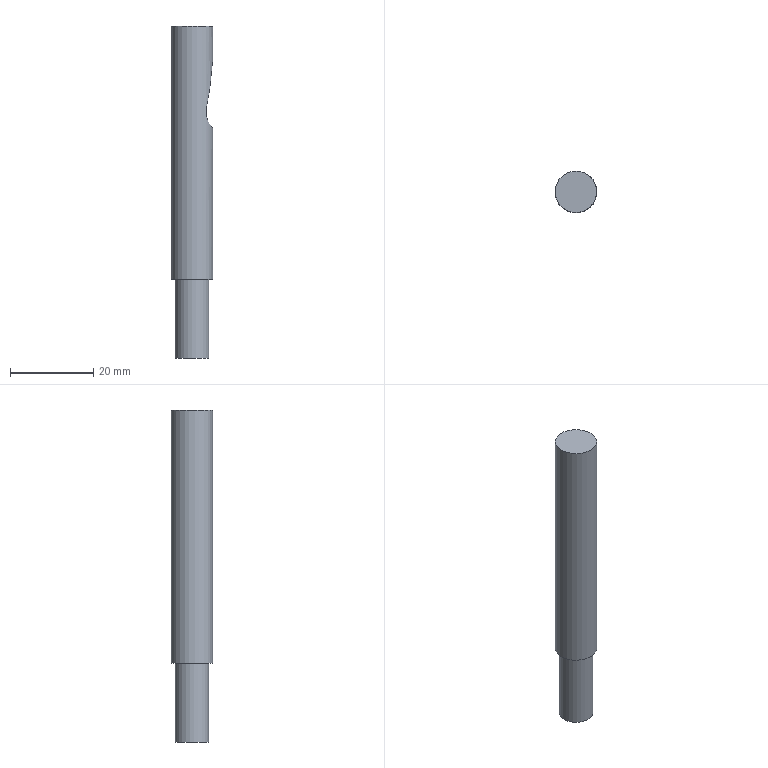Part | NX | features solid 2 | 1 solid | 8 faces | volume 5592 mm3 | plane 3 | cylinder 2 | sphere 2 | cone 1 | commonest cylinder face diameters 8.1 x1 10 x1